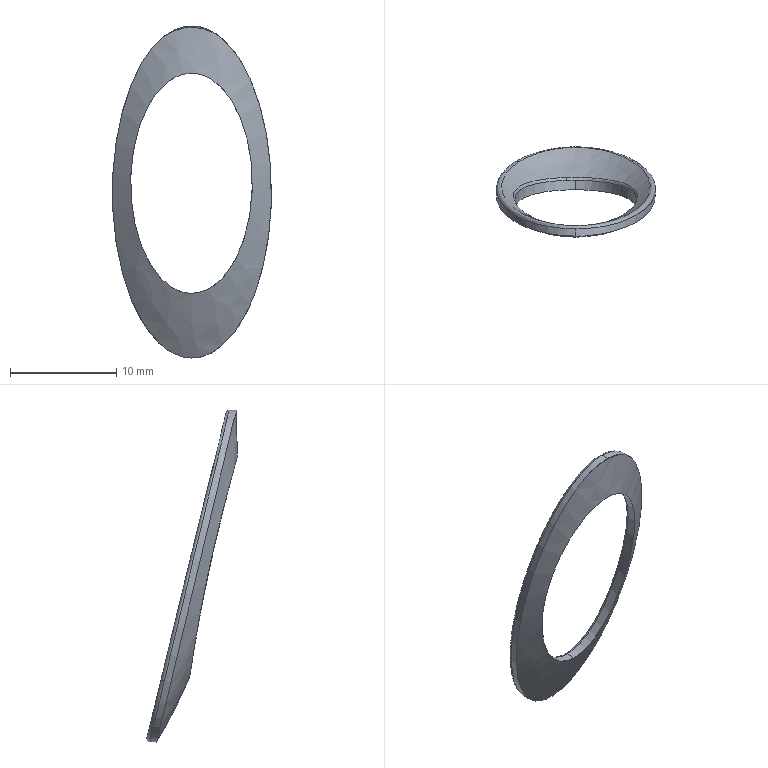Part | STEP file | Guide wheel mechanism revised.sldasm-Part-307 | 1 solid | 11 faces | volume 200.153 mm3 | spline 11